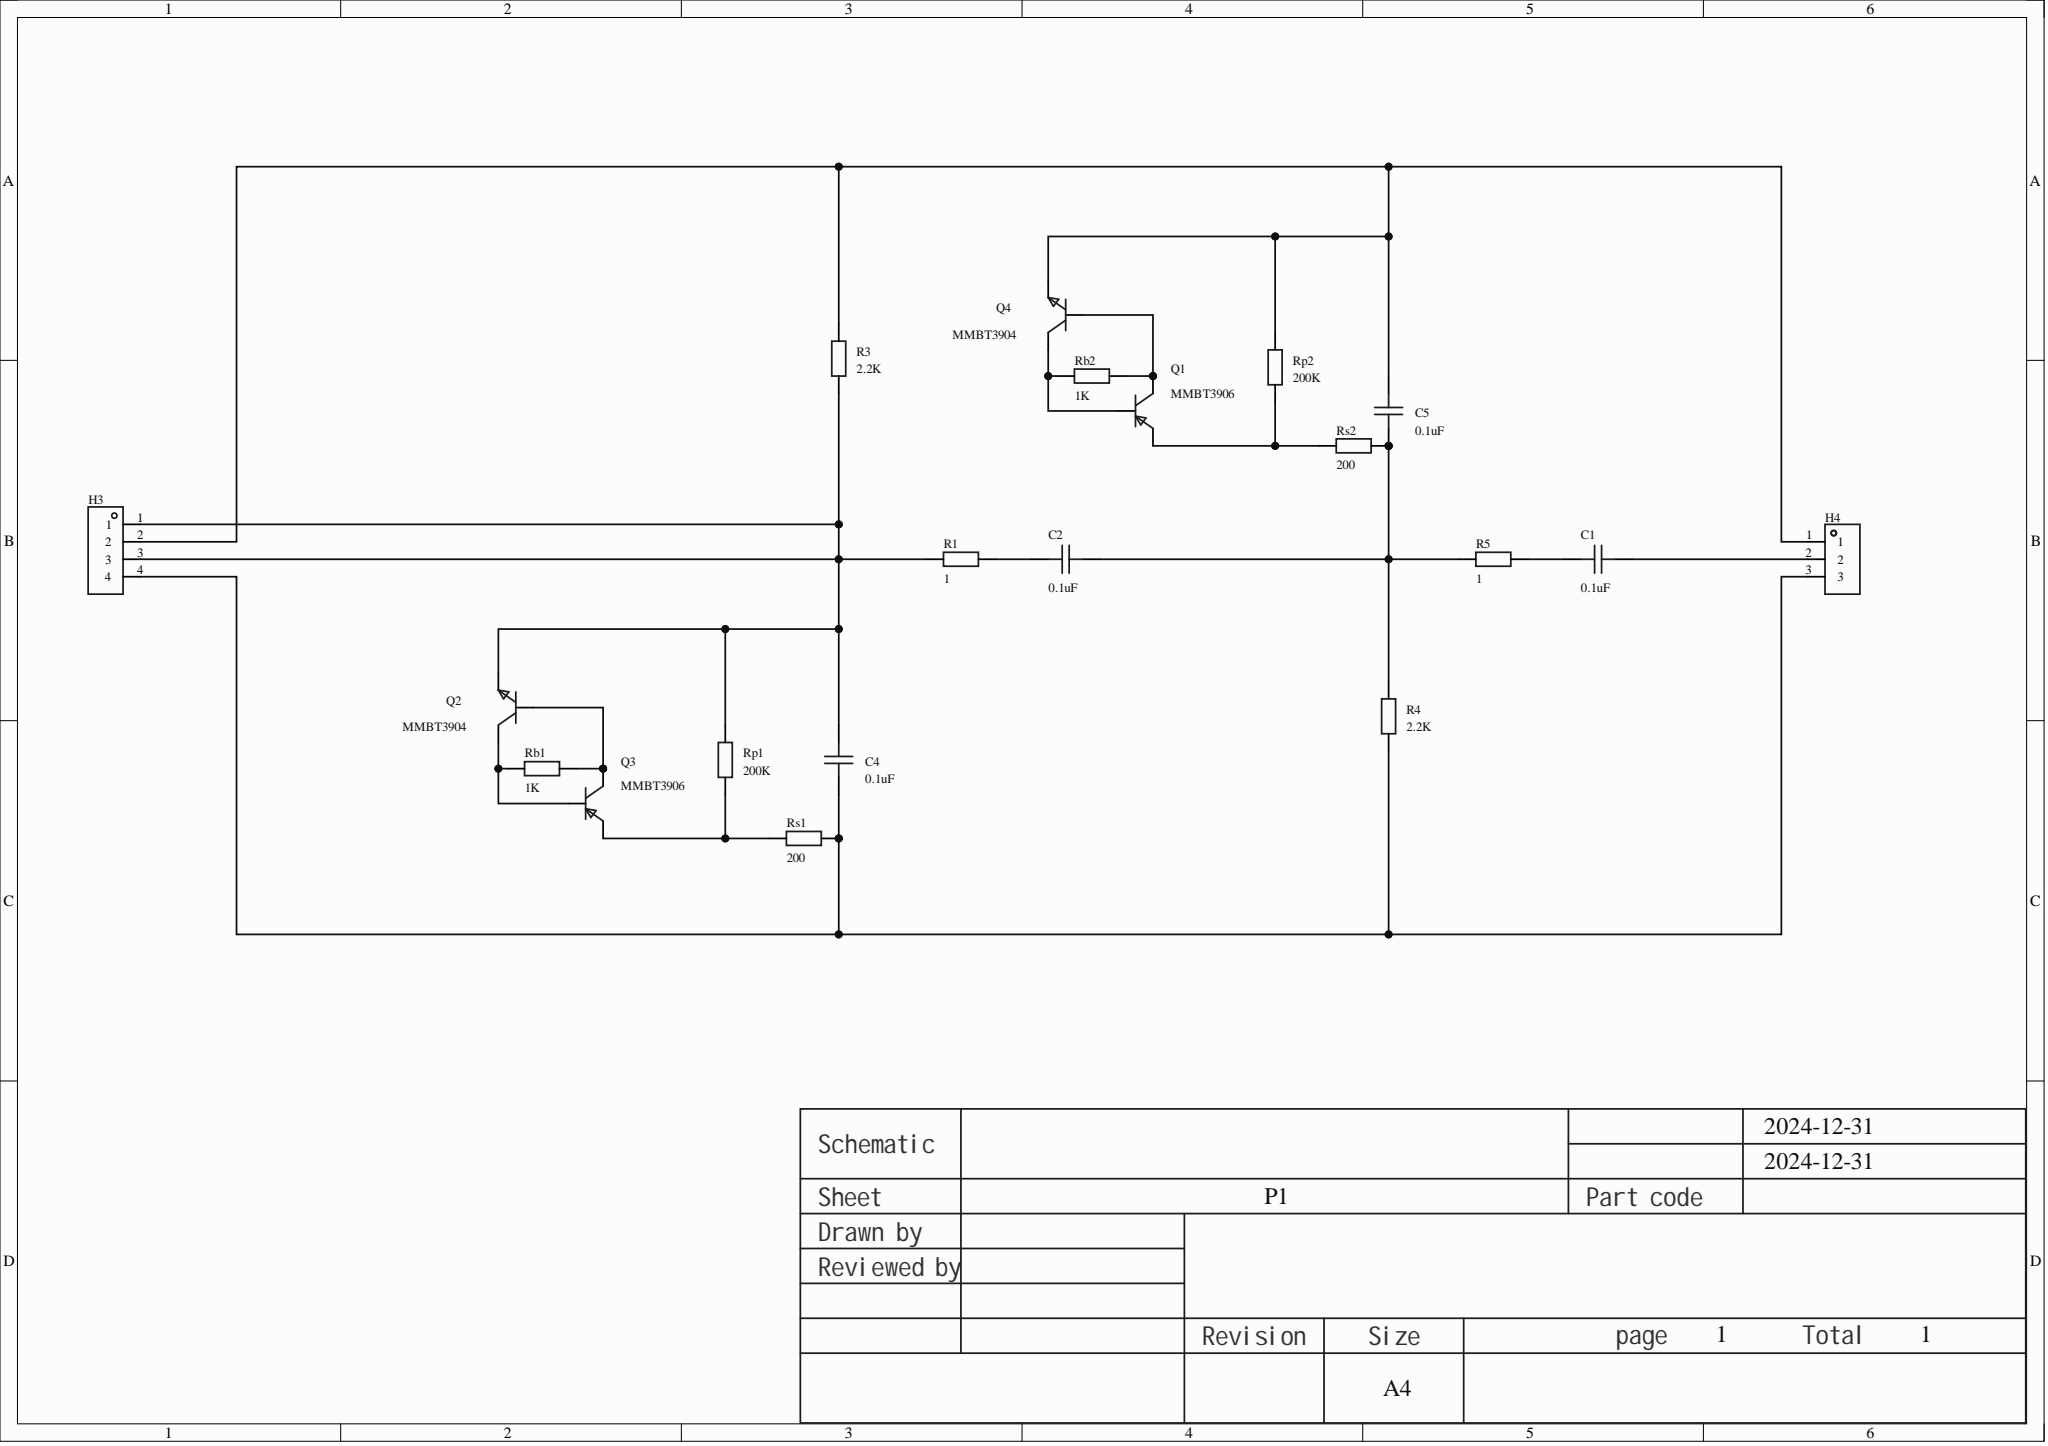Circuit board | Altium Designer | 20 parts | 13 nets
Bill of materials:
Comment,Description,Designator,Footprint,LibRef,Quantity
"0.1uF","","C1, C2, C4, C5","C0402","CAP_0402","4"
"","","H3","HDR-TH_4P-P2.54-V-M","HDR-M_2.54_1x4P","1"
"","","H4","HDR-TH_3P-P2.54-V-M","HDR-M_2.54_1x3P","1"
"MMBT3906","Transistor type: -; collector current (Ic): -; collector-emitter breakdown voltage (Vceo): -; power (Pd): -;","Q1, Q3","SOT-23-3_L2.9-W1.3-P1.90-LS2.4-BR","MMBT3906-13-01-F","2"
"MMBT3904","Transistor type: NPN; collector current (Ic): 200mA; collector-emitter breakdown voltage (Vceo): 40V; power (Pd): 200mW; DC current gain (hFE@Ic,Vce): 100@10mA,1V;","Q2, Q4","SOT-23-3_L2.9-W1.3-P1.90-LS2.4-BR","MMBT3904(RANGE:100-300)","2"
"1","","R1, R5","R0402","Res_0402","2"
"2.2K","","R3, R4","R0402","Res_0402","2"
"1K","","Rb1, Rb2","R0402","Res_0402","2"
"200K","","Rp1, Rp2","R0402","Res_0402","2"
"200","","Rs1, Rs2","R0402","Res_0402","2"
Netlist (Protel format):
[
C1
C0402
0.1uF



]
[
C2
C0402
0.1uF



]
[
C4
C0402
0.1uF



]
[
C5
C0402
0.1uF



]
[
H3
HDR-TH_4P-P2.54-V-M




]
[
H4
HDR-TH_3P-P2.54-V-M




]
[
Q1
SOT-23-3_L2.9-W1.3-P1.90-LS2.4-BR
MMBT3906



]
[
Q2
SOT-23-3_L2.9-W1.3-P1.90-LS2.4-BR
MMBT3904



]
[
Q3
SOT-23-3_L2.9-W1.3-P1.90-LS2.4-BR
MMBT3906



]
[
Q4
SOT-23-3_L2.9-W1.3-P1.90-LS2.4-BR
MMBT3904



]
[
R1
R0402
1



]
[
R3
R0402
2.2K



]
[
R4
R0402
2.2K



]
[
R5
R0402
1



]
[
Rb1
R0402
1K



]
[
Rb2
R0402
1K



]
[
Rp1
R0402
200K



]
[
Rp2
R0402
200K



]
[
Rs1
R0402
200



]
[
Rs2
R0402
200



]
(
NetQ3_2
Q3-2
Rp1-1
Rs1-1
)
(
NetQ2_3
Q2-3
Q3-1
Rb1-2
)
(
NetQ2_1
Q2-1
Q3-3
Rb1-1
)
(
NetQ1_3
Q1-3
Q4-1
Rb2-1
)
(
NetQ1_2
Q1-2
Rp2-1
Rs2-1
)
(
NetQ1_1
Q1-1
Q4-3
Rb2-2
)
(
NetC5_2
C5-2
H3-2
H4-1
Q4-2
R3-2
Rp2-2
)
(
NetC4_2
C4-2
H3-1
H3-3
Q2-2
R1-2
R3-1
Rp1-2
)
(
NetC4_1
C4-1
H3-4
H4-3
R4-1
Rs1-2
)
(
NetC2_2
C2-2
R1-1
)
(
NetC2_1
C2-1
C5-1
R4-2
R5-2
Rs2-2
)
(
NetC1_2
C1-2
R5-1
)
(
NetC1_1
C1-1
H4-2
)